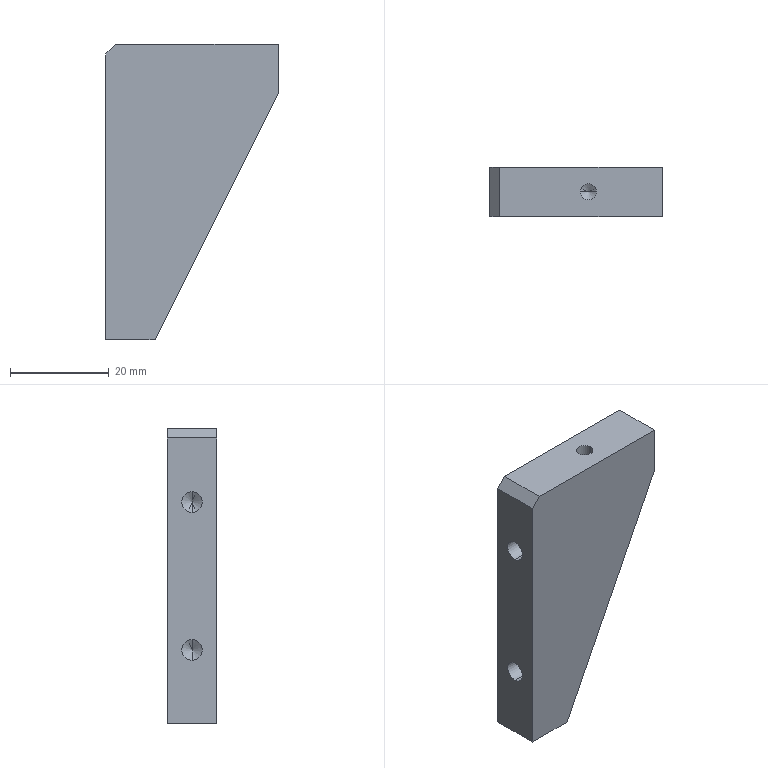Part | STEP file | PN_0051 | 1 solid | 20 faces | box 35 x 10 x 60 mm | volume 14229 mm3 | plane 8 | cylinder 6 | cone 6 | commonest cylinder face diameters 4.2 x4 3.3 x2
STEP:
#1=CARTESIAN_POINT('',(0.,0.,0.));
#2=DIRECTION('',(0.,0.,1.));
#3=DIRECTION('',(1.,0.,0.));
#4=AXIS2_PLACEMENT_3D('',#1,#2,#3);
#5=CARTESIAN_POINT('',(21.65,5.,-11.5));
#6=VERTEX_POINT('',#5);
#7=CARTESIAN_POINT('',(21.65,5.,0.));
#8=VERTEX_POINT('',#7);
#9=CARTESIAN_POINT('',(21.65,5.,0.));
#10=DIRECTION('',(0.,0.,1.));
#11=VECTOR('',#10,1.);
#12=LINE('',#9,#11);
#13=CARTESIAN_POINT('',(20.,5.,0.));
#14=DIRECTION('',(0.,0.,1.));
#15=DIRECTION('',(1.,0.,0.));
#16=AXIS2_PLACEMENT_3D('',#13,#14,#15);
#17=CYLINDRICAL_SURFACE('',#16,1.65);
#18=CARTESIAN_POINT('',(6.283,0.));
#19=DIRECTION('',(0.,1.));
#20=VECTOR('',#19,1.);
#21=LINE('',#18,#20);
#22=(GEOMETRIC_REPRESENTATION_CONTEXT(2)PARAMETRIC_REPRESENTATION_CONTEXT()REPRESENTATION_CONTEXT('',''));
#23=DEFINITIONAL_REPRESENTATION('',(#21),#22);
#24=PCURVE('',#17,#23);
#25=CARTESIAN_POINT('',(20.,5.,0.));
#26=DIRECTION('',(0.,0.,1.));
#27=DIRECTION('',(1.,0.,0.));
#28=AXIS2_PLACEMENT_3D('',#25,#26,#27);
#29=CYLINDRICAL_SURFACE('',#28,1.65);
#30=CARTESIAN_POINT('',(0.,0.));
#31=DIRECTION('',(0.,1.));
#32=VECTOR('',#31,1.);
#33=LINE('',#30,#32);
#34=(GEOMETRIC_REPRESENTATION_CONTEXT(2)PARAMETRIC_REPRESENTATION_CONTEXT()REPRESENTATION_CONTEXT('',''));
#35=DEFINITIONAL_REPRESENTATION('',(#33),#34);
#36=PCURVE('',#29,#35);
#37=SURFACE_CURVE('',#12,(#24,#36),.PCURVE_S1.);
#38=EDGE_CURVE('',#6,#8,#37,.T.);
#39=ORIENTED_EDGE('',*,*,#38,.T.);
#40=CARTESIAN_POINT('',(18.35,5.,0.));
#41=VERTEX_POINT('',#40);
#42=CARTESIAN_POINT('',(20.,5.,0.));
#43=DIRECTION('',(0.,0.,1.));
#44=DIRECTION('',(1.,0.,0.));
#45=AXIS2_PLACEMENT_3D('',#42,#43,#44);
#46=CIRCLE('',#45,1.65);
#47=CARTESIAN_POINT('',(0.,0.));
#48=DIRECTION('',(1.,0.));
#49=VECTOR('',#48,1.);
#50=LINE('',#47,#49);
#51=(GEOMETRIC_REPRESENTATION_CONTEXT(2)PARAMETRIC_REPRESENTATION_CONTEXT()REPRESENTATION_CONTEXT('',''));
#52=DEFINITIONAL_REPRESENTATION('',(#50),#51);
#53=PCURVE('',#17,#52);
#54=CARTESIAN_POINT('',(0.,10.,0.));
#55=DIRECTION('',(0.,0.,-1.));
#56=DIRECTION('',(-1.,0.,0.));
#57=AXIS2_PLACEMENT_3D('',#54,#55,#56);
#58=PLANE('',#57);
#59=CARTESIAN_POINT('',(-21.65,-5.));
#60=CARTESIAN_POINT('',(-21.65,-2.142));
#61=CARTESIAN_POINT('',(-19.175,-3.571));
#62=CARTESIAN_POINT('',(-16.7,-5.));
#63=CARTESIAN_POINT('',(-19.175,-6.429));
#64=CARTESIAN_POINT('',(-21.65,-7.858));
#65=CARTESIAN_POINT('',(-21.65,-5.));
#66=(BOUNDED_CURVE()B_SPLINE_CURVE(2,(#59,#60,#61,#62,#63,#64,#65),.UNSPECIFIED.,.T.,.F.)B_SPLINE_CURVE_WITH_KNOTS((1,2,2,2,2,1),(-2.094,0.,2.094,4.189,6.283,8.378),.UNSPECIFIED.)CURVE()GEOMETRIC_REPRESENTATION_ITEM()RATIONAL_B_SPLINE_CURVE((1.,0.5,1.,0.5,1.,0.5,1.))REPRESENTATION_ITEM(''));
#67=(GEOMETRIC_REPRESENTATION_CONTEXT(2)PARAMETRIC_REPRESENTATION_CONTEXT()REPRESENTATION_CONTEXT('',''));
#68=DEFINITIONAL_REPRESENTATION('',(#66),#67);
#69=PCURVE('',#58,#68);
#70=SURFACE_CURVE('',#46,(#53,#69),.PCURVE_S1.);
#71=EDGE_CURVE('',#41,#8,#70,.T.);
#72=ORIENTED_EDGE('',*,*,#71,.F.);
#73=CARTESIAN_POINT('',(18.35,5.,-11.5));
#74=VERTEX_POINT('',#73);
#75=CARTESIAN_POINT('',(18.35,5.,0.));
#76=DIRECTION('',(0.,0.,1.));
#77=VECTOR('',#76,1.);
#78=LINE('',#75,#77);
#79=CARTESIAN_POINT('',(3.142,0.));
#80=DIRECTION('',(0.,1.));
#81=VECTOR('',#80,1.);
#82=LINE('',#79,#81);
#83=(GEOMETRIC_REPRESENTATION_CONTEXT(2)PARAMETRIC_REPRESENTATION_CONTEXT()REPRESENTATION_CONTEXT('',''));
#84=DEFINITIONAL_REPRESENTATION('',(#82),#83);
#85=PCURVE('',#17,#84);
#86=CARTESIAN_POINT('',(3.142,0.));
#87=DIRECTION('',(0.,1.));
#88=VECTOR('',#87,1.);
#89=LINE('',#86,#88);
#90=(GEOMETRIC_REPRESENTATION_CONTEXT(2)PARAMETRIC_REPRESENTATION_CONTEXT()REPRESENTATION_CONTEXT('',''));
#91=DEFINITIONAL_REPRESENTATION('',(#89),#90);
#92=PCURVE('',#29,#91);
#93=SURFACE_CURVE('',#78,(#85,#92),.PCURVE_S1.);
#94=EDGE_CURVE('',#74,#41,#93,.T.);
#95=ORIENTED_EDGE('',*,*,#94,.F.);
#96=CARTESIAN_POINT('',(20.,5.,-11.5));
#97=DIRECTION('',(0.,0.,1.));
#98=DIRECTION('',(1.,0.,0.));
#99=AXIS2_PLACEMENT_3D('',#96,#97,#98);
#100=CIRCLE('',#99,1.65);
#101=CARTESIAN_POINT('',(0.,-11.5));
#102=DIRECTION('',(1.,0.));
#103=VECTOR('',#102,1.);
#104=LINE('',#101,#103);
#105=(GEOMETRIC_REPRESENTATION_CONTEXT(2)PARAMETRIC_REPRESENTATION_CONTEXT()REPRESENTATION_CONTEXT('',''));
#106=DEFINITIONAL_REPRESENTATION('',(#104),#105);
#107=PCURVE('',#17,#106);
#108=CARTESIAN_POINT('',(20.,5.,-11.5));
#109=DIRECTION('',(0.,0.,1.));
#110=DIRECTION('',(1.,0.,0.));
#111=AXIS2_PLACEMENT_3D('',#108,#109,#110);
#112=CONICAL_SURFACE('',#111,1.65,1.03);
#113=CARTESIAN_POINT('',(0.,0.));
#114=DIRECTION('',(1.,0.));
#115=VECTOR('',#114,1.);
#116=LINE('',#113,#115);
#117=(GEOMETRIC_REPRESENTATION_CONTEXT(2)PARAMETRIC_REPRESENTATION_CONTEXT()REPRESENTATION_CONTEXT('',''));
#118=DEFINITIONAL_REPRESENTATION('',(#116),#117);
#119=PCURVE('',#112,#118);
#120=SURFACE_CURVE('',#100,(#107,#119),.PCURVE_S1.);
#121=EDGE_CURVE('',#74,#6,#120,.T.);
#122=ORIENTED_EDGE('',*,*,#121,.T.);
#123=EDGE_LOOP('',(#39,#72,#95,#122));
#124=FACE_BOUND('',#123,.F.);
#125=ADVANCED_FACE('',(#124),#17,.F.);
#126=ORIENTED_EDGE('',*,*,#121,.F.);
#127=CARTESIAN_POINT('',(20.,5.,-12.491));
#128=VERTEX_POINT('',#127);
#129=CARTESIAN_POINT('',(18.35,5.,-11.5));
#130=DIRECTION('',(-0.8572,0.,0.515));
#131=VECTOR('',#130,1.);
#132=LINE('',#129,#131);
#133=CARTESIAN_POINT('',(3.142,0.));
#134=DIRECTION('',(0.,1.));
#135=VECTOR('',#134,1.);
#136=LINE('',#133,#135);
#137=(GEOMETRIC_REPRESENTATION_CONTEXT(2)PARAMETRIC_REPRESENTATION_CONTEXT()REPRESENTATION_CONTEXT('',''));
#138=DEFINITIONAL_REPRESENTATION('',(#136),#137);
#139=PCURVE('',#112,#138);
#140=CARTESIAN_POINT('',(20.,5.,-11.5));
#141=DIRECTION('',(0.,0.,1.));
#142=DIRECTION('',(1.,0.,0.));
#143=AXIS2_PLACEMENT_3D('',#140,#141,#142);
#144=CONICAL_SURFACE('',#143,1.65,1.03);
#145=CARTESIAN_POINT('',(3.142,0.));
#146=DIRECTION('',(0.,1.));
#147=VECTOR('',#146,1.);
#148=LINE('',#145,#147);
#149=(GEOMETRIC_REPRESENTATION_CONTEXT(2)PARAMETRIC_REPRESENTATION_CONTEXT()REPRESENTATION_CONTEXT('',''));
#150=DEFINITIONAL_REPRESENTATION('',(#148),#149);
#151=PCURVE('',#144,#150);
#152=SURFACE_CURVE('',#132,(#139,#151),.PCURVE_S1.);
#153=EDGE_CURVE('',#128,#74,#152,.T.);
#154=ORIENTED_EDGE('',*,*,#153,.F.);
#155=CARTESIAN_POINT('',(21.65,5.,-11.5));
#156=DIRECTION('',(0.8572,0.,0.515));
#157=VECTOR('',#156,1.);
#158=LINE('',#155,#157);
#159=CARTESIAN_POINT('',(6.283,0.));
#160=DIRECTION('',(0.,1.));
#161=VECTOR('',#160,1.);
#162=LINE('',#159,#161);
#163=(GEOMETRIC_REPRESENTATION_CONTEXT(2)PARAMETRIC_REPRESENTATION_CONTEXT()REPRESENTATION_CONTEXT('',''));
#164=DEFINITIONAL_REPRESENTATION('',(#162),#163);
#165=PCURVE('',#112,#164);
#166=CARTESIAN_POINT('',(0.,0.));
#167=DIRECTION('',(0.,1.));
#168=VECTOR('',#167,1.);
#169=LINE('',#166,#168);
#170=(GEOMETRIC_REPRESENTATION_CONTEXT(2)PARAMETRIC_REPRESENTATION_CONTEXT()REPRESENTATION_CONTEXT('',''));
#171=DEFINITIONAL_REPRESENTATION('',(#169),#170);
#172=PCURVE('',#144,#171);
#173=SURFACE_CURVE('',#158,(#165,#172),.PCURVE_S1.);
#174=EDGE_CURVE('',#128,#6,#173,.T.);
#175=ORIENTED_EDGE('',*,*,#174,.T.);
#176=EDGE_LOOP('',(#126,#154,#175));
#177=FACE_BOUND('',#176,.F.);
#178=ADVANCED_FACE('',(#177),#112,.F.);
#179=CARTESIAN_POINT('',(14.,5.,-42.9));
#180=VERTEX_POINT('',#179);
#181=CARTESIAN_POINT('',(0.,5.,-42.9));
#182=VERTEX_POINT('',#181);
#183=CARTESIAN_POINT('',(0.,5.,-42.9));
#184=DIRECTION('',(-1.,0.,0.));
#185=VECTOR('',#184,1.);
#186=LINE('',#183,#185);
#187=CARTESIAN_POINT('',(0.,5.,-45.));
#188=DIRECTION('',(-1.,0.,0.));
#189=DIRECTION('',(0.,0.,1.));
#190=AXIS2_PLACEMENT_3D('',#187,#188,#189);
#191=CYLINDRICAL_SURFACE('',#190,2.1);
#192=CARTESIAN_POINT('',(6.283,0.));
#193=DIRECTION('',(0.,1.));
#194=VECTOR('',#193,1.);
#195=LINE('',#192,#194);
#196=(GEOMETRIC_REPRESENTATION_CONTEXT(2)PARAMETRIC_REPRESENTATION_CONTEXT()REPRESENTATION_CONTEXT('',''));
#197=DEFINITIONAL_REPRESENTATION('',(#195),#196);
#198=PCURVE('',#191,#197);
#199=CARTESIAN_POINT('',(0.,5.,-45.));
#200=DIRECTION('',(-1.,0.,0.));
#201=DIRECTION('',(0.,0.,1.));
#202=AXIS2_PLACEMENT_3D('',#199,#200,#201);
#203=CYLINDRICAL_SURFACE('',#202,2.1);
#204=CARTESIAN_POINT('',(0.,0.));
#205=DIRECTION('',(0.,1.));
#206=VECTOR('',#205,1.);
#207=LINE('',#204,#206);
#208=(GEOMETRIC_REPRESENTATION_CONTEXT(2)PARAMETRIC_REPRESENTATION_CONTEXT()REPRESENTATION_CONTEXT('',''));
#209=DEFINITIONAL_REPRESENTATION('',(#207),#208);
#210=PCURVE('',#203,#209);
#211=SURFACE_CURVE('',#186,(#198,#210),.PCURVE_S1.);
#212=EDGE_CURVE('',#180,#182,#211,.T.);
#213=ORIENTED_EDGE('',*,*,#212,.T.);
#214=CARTESIAN_POINT('',(0.,5.,-47.1));
#215=VERTEX_POINT('',#214);
#216=CARTESIAN_POINT('',(0.,5.,-45.));
#217=DIRECTION('',(-1.,0.,0.));
#218=DIRECTION('',(0.,0.,1.));
#219=AXIS2_PLACEMENT_3D('',#216,#217,#218);
#220=CIRCLE('',#219,2.1);
#221=CARTESIAN_POINT('',(0.,0.));
#222=DIRECTION('',(1.,0.));
#223=VECTOR('',#222,1.);
#224=LINE('',#221,#223);
#225=(GEOMETRIC_REPRESENTATION_CONTEXT(2)PARAMETRIC_REPRESENTATION_CONTEXT()REPRESENTATION_CONTEXT('',''));
#226=DEFINITIONAL_REPRESENTATION('',(#224),#225);
#227=PCURVE('',#191,#226);
#228=CARTESIAN_POINT('',(0.,10.,-60.));
#229=DIRECTION('',(1.,0.,0.));
#230=DIRECTION('',(0.,0.,-1.));
#231=AXIS2_PLACEMENT_3D('',#228,#229,#230);
#232=PLANE('',#231);
#233=CARTESIAN_POINT('',(-17.1,-5.));
#234=CARTESIAN_POINT('',(-17.1,-1.363));
#235=CARTESIAN_POINT('',(-13.95,-3.181));
#236=CARTESIAN_POINT('',(-10.8,-5.));
#237=CARTESIAN_POINT('',(-13.95,-6.819));
#238=CARTESIAN_POINT('',(-17.1,-8.637));
#239=CARTESIAN_POINT('',(-17.1,-5.));
#240=(BOUNDED_CURVE()B_SPLINE_CURVE(2,(#233,#234,#235,#236,#237,#238,#239),.UNSPECIFIED.,.T.,.F.)B_SPLINE_CURVE_WITH_KNOTS((1,2,2,2,2,1),(-2.094,0.,2.094,4.189,6.283,8.378),.UNSPECIFIED.)CURVE()GEOMETRIC_REPRESENTATION_ITEM()RATIONAL_B_SPLINE_CURVE((1.,0.5,1.,0.5,1.,0.5,1.))REPRESENTATION_ITEM(''));
#241=(GEOMETRIC_REPRESENTATION_CONTEXT(2)PARAMETRIC_REPRESENTATION_CONTEXT()REPRESENTATION_CONTEXT('',''));
#242=DEFINITIONAL_REPRESENTATION('',(#240),#241);
#243=PCURVE('',#232,#242);
#244=SURFACE_CURVE('',#220,(#227,#243),.PCURVE_S1.);
#245=EDGE_CURVE('',#215,#182,#244,.T.);
#246=ORIENTED_EDGE('',*,*,#245,.F.);
#247=CARTESIAN_POINT('',(14.,5.,-47.1));
#248=VERTEX_POINT('',#247);
#249=CARTESIAN_POINT('',(0.,5.,-47.1));
#250=DIRECTION('',(-1.,0.,0.));
#251=VECTOR('',#250,1.);
#252=LINE('',#249,#251);
#253=CARTESIAN_POINT('',(3.142,0.));
#254=DIRECTION('',(0.,1.));
#255=VECTOR('',#254,1.);
#256=LINE('',#253,#255);
#257=(GEOMETRIC_REPRESENTATION_CONTEXT(2)PARAMETRIC_REPRESENTATION_CONTEXT()REPRESENTATION_CONTEXT('',''));
#258=DEFINITIONAL_REPRESENTATION('',(#256),#257);
#259=PCURVE('',#191,#258);
#260=CARTESIAN_POINT('',(3.142,0.));
#261=DIRECTION('',(0.,1.));
#262=VECTOR('',#261,1.);
#263=LINE('',#260,#262);
#264=(GEOMETRIC_REPRESENTATION_CONTEXT(2)PARAMETRIC_REPRESENTATION_CONTEXT()REPRESENTATION_CONTEXT('',''));
#265=DEFINITIONAL_REPRESENTATION('',(#263),#264);
#266=PCURVE('',#203,#265);
#267=SURFACE_CURVE('',#252,(#259,#266),.PCURVE_S1.);
#268=EDGE_CURVE('',#248,#215,#267,.T.);
#269=ORIENTED_EDGE('',*,*,#268,.F.);
#270=CARTESIAN_POINT('',(14.,5.,-45.));
#271=DIRECTION('',(-1.,0.,0.));
#272=DIRECTION('',(0.,0.,1.));
#273=AXIS2_PLACEMENT_3D('',#270,#271,#272);
#274=CIRCLE('',#273,2.1);
#275=CARTESIAN_POINT('',(0.,-14.));
#276=DIRECTION('',(1.,0.));
#277=VECTOR('',#276,1.);
#278=LINE('',#275,#277);
#279=(GEOMETRIC_REPRESENTATION_CONTEXT(2)PARAMETRIC_REPRESENTATION_CONTEXT()REPRESENTATION_CONTEXT('',''));
#280=DEFINITIONAL_REPRESENTATION('',(#278),#279);
#281=PCURVE('',#191,#280);
#282=CARTESIAN_POINT('',(14.,5.,-45.));
#283=DIRECTION('',(-1.,0.,0.));
#284=DIRECTION('',(0.,0.,1.));
#285=AXIS2_PLACEMENT_3D('',#282,#283,#284);
#286=CONICAL_SURFACE('',#285,2.1,1.03);
#287=CARTESIAN_POINT('',(0.,0.));
#288=DIRECTION('',(1.,0.));
#289=VECTOR('',#288,1.);
#290=LINE('',#287,#289);
#291=(GEOMETRIC_REPRESENTATION_CONTEXT(2)PARAMETRIC_REPRESENTATION_CONTEXT()REPRESENTATION_CONTEXT('',''));
#292=DEFINITIONAL_REPRESENTATION('',(#290),#291);
#293=PCURVE('',#286,#292);
#294=SURFACE_CURVE('',#274,(#281,#293),.PCURVE_S1.);
#295=EDGE_CURVE('',#248,#180,#294,.T.);
#296=ORIENTED_EDGE('',*,*,#295,.T.);
#297=EDGE_LOOP('',(#213,#246,#269,#296));
#298=FACE_BOUND('',#297,.F.);
#299=ADVANCED_FACE('',(#298),#191,.F.);
#300=ORIENTED_EDGE('',*,*,#295,.F.);
#301=CARTESIAN_POINT('',(15.262,5.,-45.));
#302=VERTEX_POINT('',#301);
#303=CARTESIAN_POINT('',(14.,5.,-47.1));
#304=DIRECTION('',(-0.515,0.,-0.8572));
#305=VECTOR('',#304,1.);
#306=LINE('',#303,#305);
#307=CARTESIAN_POINT('',(3.142,-1.262));
#308=CARTESIAN_POINT('',(3.142,-1.243));
#309=CARTESIAN_POINT('',(3.142,-1.204));
#310=CARTESIAN_POINT('',(3.142,-1.147));
#311=CARTESIAN_POINT('',(3.142,-1.09));
#312=CARTESIAN_POINT('',(3.142,-1.032));
#313=CARTESIAN_POINT('',(3.142,-0.975));
#314=CARTESIAN_POINT('',(3.142,-0.9177));
#315=CARTESIAN_POINT('',(3.142,-0.8603));
#316=CARTESIAN_POINT('',(3.142,-0.803));
#317=CARTESIAN_POINT('',(3.142,-0.7456));
#318=CARTESIAN_POINT('',(3.142,-0.6883));
#319=CARTESIAN_POINT('',(3.142,-0.6309));
#320=CARTESIAN_POINT('',(3.142,-0.5735));
#321=CARTESIAN_POINT('',(3.142,-0.5162));
#322=CARTESIAN_POINT('',(3.142,-0.4588));
#323=CARTESIAN_POINT('',(3.142,-0.4015));
#324=CARTESIAN_POINT('',(3.142,-0.3441));
#325=CARTESIAN_POINT('',(3.142,-0.2868));
#326=CARTESIAN_POINT('',(3.142,-0.2294));
#327=CARTESIAN_POINT('',(3.142,-0.1721));
#328=CARTESIAN_POINT('',(3.142,-0.1147));
#329=CARTESIAN_POINT('',(3.142,-0.05735));
#330=CARTESIAN_POINT('',(3.142,-0.01912));
#331=CARTESIAN_POINT('',(3.142,0.));
#332=B_SPLINE_CURVE_WITH_KNOTS('',3,(#307,#308,#309,#310,#311,#312,#313,#314,#315,#316,#317,#318,#319,#320,#321,#322,#323,#324,#325,#326,#327,#328,#329,#330,#331),.UNSPECIFIED.,.F.,.F.,(4,1,1,1,1,1,1,1,1,1,1,1,1,1,1,1,1,1,1,1,1,1,4),(-2.45,-2.339,-2.227,-2.116,-2.004,-1.893,-1.782,-1.67,-1.559,-1.448,-1.336,-1.225,-1.114,-1.002,-0.8909,-0.7795,-0.6682,-0.5568,-0.4454,-0.3341,-0.2227,-0.1114,0.),.UNSPECIFIED.);
#333=(GEOMETRIC_REPRESENTATION_CONTEXT(2)PARAMETRIC_REPRESENTATION_CONTEXT()REPRESENTATION_CONTEXT('',''));
#334=DEFINITIONAL_REPRESENTATION('',(#332),#333);
#335=PCURVE('',#286,#334);
#336=CARTESIAN_POINT('',(14.,5.,-45.));
#337=DIRECTION('',(-1.,0.,0.));
#338=DIRECTION('',(0.,0.,1.));
#339=AXIS2_PLACEMENT_3D('',#336,#337,#338);
#340=CONICAL_SURFACE('',#339,2.1,1.03);
#341=CARTESIAN_POINT('',(3.142,-1.262));
#342=CARTESIAN_POINT('',(3.142,-1.243));
#343=CARTESIAN_POINT('',(3.142,-1.204));
#344=CARTESIAN_POINT('',(3.142,-1.147));
#345=CARTESIAN_POINT('',(3.142,-1.09));
#346=CARTESIAN_POINT('',(3.142,-1.032));
#347=CARTESIAN_POINT('',(3.142,-0.975));
#348=CARTESIAN_POINT('',(3.142,-0.9177));
#349=CARTESIAN_POINT('',(3.142,-0.8603));
#350=CARTESIAN_POINT('',(3.142,-0.803));
#351=CARTESIAN_POINT('',(3.142,-0.7456));
#352=CARTESIAN_POINT('',(3.142,-0.6883));
#353=CARTESIAN_POINT('',(3.142,-0.6309));
#354=CARTESIAN_POINT('',(3.142,-0.5735));
#355=CARTESIAN_POINT('',(3.142,-0.5162));
#356=CARTESIAN_POINT('',(3.142,-0.4588));
#357=CARTESIAN_POINT('',(3.142,-0.4015));
#358=CARTESIAN_POINT('',(3.142,-0.3441));
#359=CARTESIAN_POINT('',(3.142,-0.2868));
#360=CARTESIAN_POINT('',(3.142,-0.2294));
#361=CARTESIAN_POINT('',(3.142,-0.1721));
#362=CARTESIAN_POINT('',(3.142,-0.1147));
#363=CARTESIAN_POINT('',(3.142,-0.05735));
#364=CARTESIAN_POINT('',(3.142,-0.01912));
#365=CARTESIAN_POINT('',(3.142,0.));
#366=B_SPLINE_CURVE_WITH_KNOTS('',3,(#341,#342,#343,#344,#345,#346,#347,#348,#349,#350,#351,#352,#353,#354,#355,#356,#357,#358,#359,#360,#361,#362,#363,#364,#365),.UNSPECIFIED.,.F.,.F.,(4,1,1,1,1,1,1,1,1,1,1,1,1,1,1,1,1,1,1,1,1,1,4),(-2.45,-2.339,-2.227,-2.116,-2.004,-1.893,-1.782,-1.67,-1.559,-1.448,-1.336,-1.225,-1.114,-1.002,-0.8909,-0.7795,-0.6682,-0.5568,-0.4454,-0.3341,-0.2227,-0.1114,0.),.UNSPECIFIED.);
#367=(GEOMETRIC_REPRESENTATION_CONTEXT(2)PARAMETRIC_REPRESENTATION_CONTEXT()REPRESENTATION_CONTEXT('',''));
#368=DEFINITIONAL_REPRESENTATION('',(#366),#367);
#369=PCURVE('',#340,#368);
#370=SURFACE_CURVE('',#306,(#335,#369),.PCURVE_S1.);
#371=EDGE_CURVE('',#302,#248,#370,.T.);
#372=ORIENTED_EDGE('',*,*,#371,.F.);
#373=CARTESIAN_POINT('',(14.,5.,-42.9));
#374=DIRECTION('',(-0.515,0.,0.8572));
#375=VECTOR('',#374,1.);
#376=LINE('',#373,#375);
#377=CARTESIAN_POINT('',(6.283,0.));
#378=DIRECTION('',(0.,1.));
#379=VECTOR('',#378,1.);
#380=LINE('',#377,#379);
#381=(GEOMETRIC_REPRESENTATION_CONTEXT(2)PARAMETRIC_REPRESENTATION_CONTEXT()REPRESENTATION_CONTEXT('',''));
#382=DEFINITIONAL_REPRESENTATION('',(#380),#381);
#383=PCURVE('',#286,#382);
#384=CARTESIAN_POINT('',(0.,0.));
#385=DIRECTION('',(0.,1.));
#386=VECTOR('',#385,1.);
#387=LINE('',#384,#386);
#388=(GEOMETRIC_REPRESENTATION_CONTEXT(2)PARAMETRIC_REPRESENTATION_CONTEXT()REPRESENTATION_CONTEXT('',''));
#389=DEFINITIONAL_REPRESENTATION('',(#387),#388);
#390=PCURVE('',#340,#389);
#391=SURFACE_CURVE('',#376,(#383,#390),.PCURVE_S1.);
#392=EDGE_CURVE('',#302,#180,#391,.T.);
#393=ORIENTED_EDGE('',*,*,#392,.T.);
#394=EDGE_LOOP('',(#300,#372,#393));
#395=FACE_BOUND('',#394,.F.);
#396=ADVANCED_FACE('',(#395),#286,.F.);
#397=CARTESIAN_POINT('',(14.,5.,-12.9));
#398=VERTEX_POINT('',#397);
#399=CARTESIAN_POINT('',(0.,5.,-12.9));
#400=VERTEX_POINT('',#399);
#401=CARTESIAN_POINT('',(0.,5.,-12.9));
#402=DIRECTION('',(-1.,0.,0.));
#403=VECTOR('',#402,1.);
#404=LINE('',#401,#403);
#405=CARTESIAN_POINT('',(0.,5.,-15.));
#406=DIRECTION('',(-1.,0.,0.));
#407=DIRECTION('',(0.,0.,1.));
#408=AXIS2_PLACEMENT_3D('',#405,#406,#407);
#409=CYLINDRICAL_SURFACE('',#408,2.1);
#410=CARTESIAN_POINT('',(6.283,0.));
#411=DIRECTION('',(0.,1.));
#412=VECTOR('',#411,1.);
#413=LINE('',#410,#412);
#414=(GEOMETRIC_REPRESENTATION_CONTEXT(2)PARAMETRIC_REPRESENTATION_CONTEXT()REPRESENTATION_CONTEXT('',''));
#415=DEFINITIONAL_REPRESENTATION('',(#413),#414);
#416=PCURVE('',#409,#415);
#417=CARTESIAN_POINT('',(0.,5.,-15.));
#418=DIRECTION('',(-1.,0.,0.));
#419=DIRECTION('',(0.,0.,1.));
#420=AXIS2_PLACEMENT_3D('',#417,#418,#419);
#421=CYLINDRICAL_SURFACE('',#420,2.1);
#422=CARTESIAN_POINT('',(0.,0.));
#423=DIRECTION('',(0.,1.));
#424=VECTOR('',#423,1.);
#425=LINE('',#422,#424);
#426=(GEOMETRIC_REPRESENTATION_CONTEXT(2)PARAMETRIC_REPRESENTATION_CONTEXT()REPRESENTATION_CONTEXT('',''));
#427=DEFINITIONAL_REPRESENTATION('',(#425),#426);
#428=PCURVE('',#421,#427);
#429=SURFACE_CURVE('',#404,(#416,#428),.PCURVE_S1.);
#430=EDGE_CURVE('',#398,#400,#429,.T.);
#431=ORIENTED_EDGE('',*,*,#430,.T.);
#432=CARTESIAN_POINT('',(0.,5.,-17.1));
#433=VERTEX_POINT('',#432);
#434=CARTESIAN_POINT('',(0.,5.,-15.));
#435=DIRECTION('',(-1.,0.,0.));
#436=DIRECTION('',(0.,0.,1.));
#437=AXIS2_PLACEMENT_3D('',#434,#435,#436);
#438=CIRCLE('',#437,2.1);
#439=CARTESIAN_POINT('',(0.,0.));
#440=DIRECTION('',(1.,0.));
#441=VECTOR('',#440,1.);
#442=LINE('',#439,#441);
#443=(GEOMETRIC_REPRESENTATION_CONTEXT(2)PARAMETRIC_REPRESENTATION_CONTEXT()REPRESENTATION_CONTEXT('',''));
#444=DEFINITIONAL_REPRESENTATION('',(#442),#443);
#445=PCURVE('',#409,#444);
#446=CARTESIAN_POINT('',(-47.1,-5.));
#447=CARTESIAN_POINT('',(-47.1,-1.363));
#448=CARTESIAN_POINT('',(-43.95,-3.181));
#449=CARTESIAN_POINT('',(-40.8,-5.));
#450=CARTESIAN_POINT('',(-43.95,-6.819));
#451=CARTESIAN_POINT('',(-47.1,-8.637));
#452=CARTESIAN_POINT('',(-47.1,-5.));
#453=(BOUNDED_CURVE()B_SPLINE_CURVE(2,(#446,#447,#448,#449,#450,#451,#452),.UNSPECIFIED.,.T.,.F.)B_SPLINE_CURVE_WITH_KNOTS((1,2,2,2,2,1),(-2.094,0.,2.094,4.189,6.283,8.378),.UNSPECIFIED.)CURVE()GEOMETRIC_REPRESENTATION_ITEM()RATIONAL_B_SPLINE_CURVE((1.,0.5,1.,0.5,1.,0.5,1.))REPRESENTATION_ITEM(''));
#454=(GEOMETRIC_REPRESENTATION_CONTEXT(2)PARAMETRIC_REPRESENTATION_CONTEXT()REPRESENTATION_CONTEXT('',''));
#455=DEFINITIONAL_REPRESENTATION('',(#453),#454);
#456=PCURVE('',#232,#455);
#457=SURFACE_CURVE('',#438,(#445,#456),.PCURVE_S1.);
#458=EDGE_CURVE('',#433,#400,#457,.T.);
#459=ORIENTED_EDGE('',*,*,#458,.F.);
#460=CARTESIAN_POINT('',(14.,5.,-17.1));
#461=VERTEX_POINT('',#460);
#462=CARTESIAN_POINT('',(0.,5.,-17.1));
#463=DIRECTION('',(-1.,0.,0.));
#464=VECTOR('',#463,1.);
#465=LINE('',#462,#464);
#466=CARTESIAN_POINT('',(3.142,0.));
#467=DIRECTION('',(0.,1.));
#468=VECTOR('',#467,1.);
#469=LINE('',#466,#468);
#470=(GEOMETRIC_REPRESENTATION_CONTEXT(2)PARAMETRIC_REPRESENTATION_CONTEXT()REPRESENTATION_CONTEXT('',''));
#471=DEFINITIONAL_REPRESENTATION('',(#469),#470);
#472=PCURVE('',#409,#471);
#473=CARTESIAN_POINT('',(3.142,0.));
#474=DIRECTION('',(0.,1.));
#475=VECTOR('',#474,1.);
#476=LINE('',#473,#475);
#477=(GEOMETRIC_REPRESENTATION_CONTEXT(2)PARAMETRIC_REPRESENTATION_CONTEXT()REPRESENTATION_CONTEXT('',''));
#478=DEFINITIONAL_REPRESENTATION('',(#476),#477);
#479=PCURVE('',#421,#478);
#480=SURFACE_CURVE('',#465,(#472,#479),.PCURVE_S1.);
#481=EDGE_CURVE('',#461,#433,#480,.T.);
#482=ORIENTED_EDGE('',*,*,#481,.F.);
#483=CARTESIAN_POINT('',(14.,5.,-15.));
#484=DIRECTION('',(-1.,0.,0.));
#485=DIRECTION('',(0.,0.,1.));
#486=AXIS2_PLACEMENT_3D('',#483,#484,#485);
#487=CIRCLE('',#486,2.1);
#488=CARTESIAN_POINT('',(0.,-14.));
#489=DIRECTION('',(1.,0.));
#490=VECTOR('',#489,1.);
#491=LINE('',#488,#490);
#492=(GEOMETRIC_REPRESENTATION_CONTEXT(2)PARAMETRIC_REPRESENTATION_CONTEXT()REPRESENTATION_CONTEXT('',''));
#493=DEFINITIONAL_REPRESENTATION('',(#491),#492);
#494=PCURVE('',#409,#493);
#495=CARTESIAN_POINT('',(14.,5.,-15.));
#496=DIRECTION('',(-1.,0.,0.));
#497=DIRECTION('',(0.,0.,1.));
#498=AXIS2_PLACEMENT_3D('',#495,#496,#497);
#499=CONICAL_SURFACE('',#498,2.1,1.03);
#500=CARTESIAN_POINT('',(0.,0.));
#501=DIRECTION('',(1.,0.));
#502=VECTOR('',#501,1.);
#503=LINE('',#500,#502);
#504=(GEOMETRIC_REPRESENTATION_CONTEXT(2)PARAMETRIC_REPRESENTATION_CONTEXT()REPRESENTATION_CONTEXT('',''));
#505=DEFINITIONAL_REPRESENTATION('',(#503),#504);
#506=PCURVE('',#499,#505);
#507=SURFACE_CURVE('',#487,(#494,#506),.PCURVE_S1.);
#508=EDGE_CURVE('',#461,#398,#507,.T.);
#509=ORIENTED_EDGE('',*,*,#508,.T.);
#510=EDGE_LOOP('',(#431,#459,#482,#509));
#511=FACE_BOUND('',#510,.F.);
#512=ADVANCED_FACE('',(#511),#409,.F.);
#513=ORIENTED_EDGE('',*,*,#508,.F.);
#514=CARTESIAN_POINT('',(15.262,5.,-15.));
#515=VERTEX_POINT('',#514);
#516=CARTESIAN_POINT('',(14.,5.,-17.1));
#517=DIRECTION('',(-0.515,0.,-0.8572));
#518=VECTOR('',#517,1.);
#519=LINE('',#516,#518);
#520=CARTESIAN_POINT('',(3.142,-1.262));
#521=CARTESIAN_POINT('',(3.142,-1.243));
#522=CARTESIAN_POINT('',(3.142,-1.204));
#523=CARTESIAN_POINT('',(3.142,-1.147));
#524=CARTESIAN_POINT('',(3.142,-1.09));
#525=CARTESIAN_POINT('',(3.142,-1.032));
#526=CARTESIAN_POINT('',(3.142,-0.975));
#527=CARTESIAN_POINT('',(3.142,-0.9177));
#528=CARTESIAN_POINT('',(3.142,-0.8603));
#529=CARTESIAN_POINT('',(3.142,-0.803));
#530=CARTESIAN_POINT('',(3.142,-0.7456));
#531=CARTESIAN_POINT('',(3.142,-0.6883));
#532=CARTESIAN_POINT('',(3.142,-0.6309));
#533=CARTESIAN_POINT('',(3.142,-0.5735));
#534=CARTESIAN_POINT('',(3.142,-0.5162));
#535=CARTESIAN_POINT('',(3.142,-0.4588));
#536=CARTESIAN_POINT('',(3.142,-0.4015));
#537=CARTESIAN_POINT('',(3.142,-0.3441));
#538=CARTESIAN_POINT('',(3.142,-0.2868));
#539=CARTESIAN_POINT('',(3.142,-0.2294));
#540=CARTESIAN_POINT('',(3.142,-0.1721));
#541=CARTESIAN_POINT('',(3.142,-0.1147));
#542=CARTESIAN_POINT('',(3.142,-0.05735));
#543=CARTESIAN_POINT('',(3.142,-0.01912));
#544=CARTESIAN_POINT('',(3.142,0.));
#545=B_SPLINE_CURVE_WITH_KNOTS('',3,(#520,#521,#522,#523,#524,#525,#526,#527,#528,#529,#530,#531,#532,#533,#534,#535,#536,#537,#538,#539,#540,#541,#542,#543,#544),.UNSPECIFIED.,.F.,.F.,(4,1,1,1,1,1,1,1,1,1,1,1,1,1,1,1,1,1,1,1,1,1,4),(-2.45,-2.339,-2.227,-2.116,-2.004,-1.893,-1.782,-1.67,-1.559,-1.448,-1.336,-1.225,-1.114,-1.002,-0.8909,-0.7795,-0.6682,-0.5568,-0.4454,-0.3341,-0.2227,-0.1114,0.),.UNSPECIFIED.);
#546=(GEOMETRIC_REPRESENTATION_CONTEXT(2)PARAMETRIC_REPRESENTATION_CONTEXT()REPRESENTATION_CONTEXT('',''));
#547=DEFINITIONAL_REPRESENTATION('',(#545),#546);
#548=PCURVE('',#499,#547);
#549=CARTESIAN_POINT('',(14.,5.,-15.));
#550=DIRECTION('',(-1.,0.,0.));
#551=DIRECTION('',(0.,0.,1.));
#552=AXIS2_PLACEMENT_3D('',#549,#550,#551);
#553=CONICAL_SURFACE('',#552,2.1,1.03);
#554=CARTESIAN_POINT('',(3.142,-1.262));
#555=CARTESIAN_POINT('',(3.142,-1.243));
#556=CARTESIAN_POINT('',(3.142,-1.204));
#557=CARTESIAN_POINT('',(3.142,-1.147));
#558=CARTESIAN_POINT('',(3.142,-1.09));
#559=CARTESIAN_POINT('',(3.142,-1.032));
#560=CARTESIAN_POINT('',(3.142,-0.975));
#561=CARTESIAN_POINT('',(3.142,-0.9177));
#562=CARTESIAN_POINT('',(3.142,-0.8603));
#563=CARTESIAN_POINT('',(3.142,-0.803));
#564=CARTESIAN_POINT('',(3.142,-0.7456));
#565=CARTESIAN_POINT('',(3.142,-0.6883));
#566=CARTESIAN_POINT('',(3.142,-0.6309));
#567=CARTESIAN_POINT('',(3.142,-0.5735));
#568=CARTESIAN_POINT('',(3.142,-0.5162));
#569=CARTESIAN_POINT('',(3.142,-0.4588));
#570=CARTESIAN_POINT('',(3.142,-0.4015));
#571=CARTESIAN_POINT('',(3.142,-0.3441));
#572=CARTESIAN_POINT('',(3.142,-0.2868));
#573=CARTESIAN_POINT('',(3.142,-0.2294));
#574=CARTESIAN_POINT('',(3.142,-0.1721));
#575=CARTESIAN_POINT('',(3.142,-0.1147));
#576=CARTESIAN_POINT('',(3.142,-0.05735));
#577=CARTESIAN_POINT('',(3.142,-0.01912));
#578=CARTESIAN_POINT('',(3.142,0.));
#579=B_SPLINE_CURVE_WITH_KNOTS('',3,(#554,#555,#556,#557,#558,#559,#560,#561,#562,#563,#564,#565,#566,#567,#568,#569,#570,#571,#572,#573,#574,#575,#576,#577,#578),.UNSPECIFIED.,.F.,.F.,(4,1,1,1,1,1,1,1,1,1,1,1,1,1,1,1,1,1,1,1,1,1,4),(-2.45,-2.339,-2.227,-2.116,-2.004,-1.893,-1.782,-1.67,-1.559,-1.448,-1.336,-1.225,-1.114,-1.002,-0.8909,-0.7795,-0.6682,-0.5568,-0.4454,-0.3341,-0.2227,-0.1114,0.),.UNSPECIFIED.);
#580=(GEOMETRIC_REPRESENTATION_CONTEXT(2)PARAMETRIC_REPRESENTATION_CONTEXT()REPRESENTATION_CONTEXT('',''));
#581=DEFINITIONAL_REPRESENTATION('',(#579),#580);
#582=PCURVE('',#553,#581);
#583=SURFACE_CURVE('',#519,(#548,#582),.PCURVE_S1.);
#584=EDGE_CURVE('',#515,#461,#583,.T.);
#585=ORIENTED_EDGE('',*,*,#584,.F.);
#586=CARTESIAN_POINT('',(14.,5.,-12.9));
#587=DIRECTION('',(-0.515,0.,0.8572));
#588=VECTOR('',#587,1.);
#589=LINE('',#586,#588);
#590=CARTESIAN_POINT('',(6.283,0.));
#591=DIRECTION('',(0.,1.));
#592=VECTOR('',#591,1.);
#593=LINE('',#590,#592);
#594=(GEOMETRIC_REPRESENTATION_CONTEXT(2)PARAMETRIC_REPRESENTATION_CONTEXT()REPRESENTATION_CONTEXT('',''));
#595=DEFINITIONAL_REPRESENTATION('',(#593),#594);
#596=PCURVE('',#499,#595);
#597=CARTESIAN_POINT('',(0.,0.));
#598=DIRECTION('',(0.,1.));
#599=VECTOR('',#598,1.);
#600=LINE('',#597,#599);
#601=(GEOMETRIC_REPRESENTATION_CONTEXT(2)PARAMETRIC_REPRESENTATION_CONTEXT()REPRESENTATION_CONTEXT('',''));
#602=DEFINITIONAL_REPRESENTATION('',(#600),#601);
#603=PCURVE('',#553,#602);
#604=SURFACE_CURVE('',#589,(#596,#603),.PCURVE_S1.);
#605=EDGE_CURVE('',#515,#398,#604,.T.);
#606=ORIENTED_EDGE('',*,*,#605,.T.);
#607=EDGE_LOOP('',(#513,#585,#606));
#608=FACE_BOUND('',#607,.F.);
#609=ADVANCED_FACE('',(#608),#499,.F.);
#610=CARTESIAN_POINT('',(0.,5.,-45.));
#611=DIRECTION('',(-1.,0.,0.));
#612=DIRECTION('',(0.,0.,1.));
#613=AXIS2_PLACEMENT_3D('',#610,#611,#612);
#614=CIRCLE('',#613,2.1);
#615=CARTESIAN_POINT('',(-17.1,-5.));
#616=CARTESIAN_POINT('',(-17.1,-1.363));
#617=CARTESIAN_POINT('',(-13.95,-3.181));
#618=CARTESIAN_POINT('',(-10.8,-5.));
#619=CARTESIAN_POINT('',(-13.95,-6.819));
#620=CARTESIAN_POINT('',(-17.1,-8.637));
#621=CARTESIAN_POINT('',(-17.1,-5.));
#622=(BOUNDED_CURVE()B_SPLINE_CURVE(2,(#615,#616,#617,#618,#619,#620,#621),.UNSPECIFIED.,.T.,.F.)B_SPLINE_CURVE_WITH_KNOTS((1,2,2,2,2,1),(-2.094,0.,2.094,4.189,6.283,8.378),.UNSPECIFIED.)CURVE()GEOMETRIC_REPRESENTATION_ITEM()RATIONAL_B_SPLINE_CURVE((1.,0.5,1.,0.5,1.,0.5,1.))REPRESENTATION_ITEM(''));
#623=(GEOMETRIC_REPRESENTATION_CONTEXT(2)PARAMETRIC_REPRESENTATION_CONTEXT()REPRESENTATION_CONTEXT('',''));
#624=DEFINITIONAL_REPRESENTATION('',(#622),#623);
#625=PCURVE('',#232,#624);
#626=CARTESIAN_POINT('',(0.,0.));
#627=DIRECTION('',(1.,0.));
#628=VECTOR('',#627,1.);
#629=LINE('',#626,#628);
#630=(GEOMETRIC_REPRESENTATION_CONTEXT(2)PARAMETRIC_REPRESENTATION_CONTEXT()REPRESENTATION_CONTEXT('',''));
#631=DEFINITIONAL_REPRESENTATION('',(#629),#630);
#632=PCURVE('',#203,#631);
#633=SURFACE_CURVE('',#614,(#625,#632),.PCURVE_S1.);
#634=EDGE_CURVE('',#182,#215,#633,.T.);
#635=ORIENTED_EDGE('',*,*,#634,.F.);
#636=ORIENTED_EDGE('',*,*,#245,.F.);
#637=EDGE_LOOP('',(#635,#636));
#638=FACE_BOUND('',#637,.T.);
#639=CARTESIAN_POINT('',(0.,5.,-15.));
#640=DIRECTION('',(-1.,0.,0.));
#641=DIRECTION('',(0.,0.,1.));
#642=AXIS2_PLACEMENT_3D('',#639,#640,#641);
#643=CIRCLE('',#642,2.1);
#644=CARTESIAN_POINT('',(-47.1,-5.));
#645=CARTESIAN_POINT('',(-47.1,-1.363));
#646=CARTESIAN_POINT('',(-43.95,-3.181));
#647=CARTESIAN_POINT('',(-40.8,-5.));
#648=CARTESIAN_POINT('',(-43.95,-6.819));
#649=CARTESIAN_POINT('',(-47.1,-8.637));
#650=CARTESIAN_POINT('',(-47.1,-5.));
#651=(BOUNDED_CURVE()B_SPLINE_CURVE(2,(#644,#645,#646,#647,#648,#649,#650),.UNSPECIFIED.,.T.,.F.)B_SPLINE_CURVE_WITH_KNOTS((1,2,2,2,2,1),(-2.094,0.,2.094,4.189,6.283,8.378),.UNSPECIFIED.)CURVE()GEOMETRIC_REPRESENTATION_ITEM()RATIONAL_B_SPLINE_CURVE((1.,0.5,1.,0.5,1.,0.5,1.))REPRESENTATION_ITEM(''));
#652=(GEOMETRIC_REPRESENTATION_CONTEXT(2)PARAMETRIC_REPRESENTATION_CONTEXT()REPRESENTATION_CONTEXT('',''));
#653=DEFINITIONAL_REPRESENTATION('',(#651),#652);
#654=PCURVE('',#232,#653);
#655=CARTESIAN_POINT('',(0.,0.));
#656=DIRECTION('',(1.,0.));
#657=VECTOR('',#656,1.);
#658=LINE('',#655,#657);
#659=(GEOMETRIC_REPRESENTATION_CONTEXT(2)PARAMETRIC_REPRESENTATION_CONTEXT()REPRESENTATION_CONTEXT('',''));
#660=DEFINITIONAL_REPRESENTATION('',(#658),#659);
#661=PCURVE('',#421,#660);
#662=SURFACE_CURVE('',#643,(#654,#661),.PCURVE_S1.);
#663=EDGE_CURVE('',#400,#433,#662,.T.);
#664=ORIENTED_EDGE('',*,*,#663,.F.);
#665=ORIENTED_EDGE('',*,*,#458,.F.);
#666=EDGE_LOOP('',(#664,#665));
#667=FACE_BOUND('',#666,.T.);
#668=CARTESIAN_POINT('',(0.,0.,-60.));
#669=VERTEX_POINT('',#668);
#670=CARTESIAN_POINT('',(0.,0.,-2.));
#671=VERTEX_POINT('',#670);
#672=CARTESIAN_POINT('',(0.,0.,-60.));
#673=DIRECTION('',(0.,0.,1.));
#674=VECTOR('',#673,1.);
#675=LINE('',#672,#674);
#676=CARTESIAN_POINT('',(0.,-10.));
#677=DIRECTION('',(-1.,0.));
#678=VECTOR('',#677,1.);
#679=LINE('',#676,#678);
#680=(GEOMETRIC_REPRESENTATION_CONTEXT(2)PARAMETRIC_REPRESENTATION_CONTEXT()REPRESENTATION_CONTEXT('',''));
#681=DEFINITIONAL_REPRESENTATION('',(#679),#680);
#682=PCURVE('',#232,#681);
#683=CARTESIAN_POINT('',(0.,0.,0.));
#684=DIRECTION('',(0.,1.,0.));
#685=DIRECTION('',(0.,0.,1.));
#686=AXIS2_PLACEMENT_3D('',#683,#684,#685);
#687=PLANE('',#686);
#688=CARTESIAN_POINT('',(-60.,0.));
#689=DIRECTION('',(1.,0.));
#690=VECTOR('',#689,1.);
#691=LINE('',#688,#690);
#692=(GEOMETRIC_REPRESENTATION_CONTEXT(2)PARAMETRIC_REPRESENTATION_CONTEXT()REPRESENTATION_CONTEXT('',''));
#693=DEFINITIONAL_REPRESENTATION('',(#691),#692);
#694=PCURVE('',#687,#693);
#695=SURFACE_CURVE('',#675,(#682,#694),.PCURVE_S1.);
#696=EDGE_CURVE('',#669,#671,#695,.T.);
#697=ORIENTED_EDGE('',*,*,#696,.T.);
#698=CARTESIAN_POINT('',(0.,10.,-2.));
#699=VERTEX_POINT('',#698);
#700=CARTESIAN_POINT('',(0.,10.,-2.));
#701=DIRECTION('',(0.,1.,0.));
#702=VECTOR('',#701,1.);
#703=LINE('',#700,#702);
#704=CARTESIAN_POINT('',(-58.,0.));
#705=DIRECTION('',(0.,1.));
#706=VECTOR('',#705,1.);
#707=LINE('',#704,#706);
#708=(GEOMETRIC_REPRESENTATION_CONTEXT(2)PARAMETRIC_REPRESENTATION_CONTEXT()REPRESENTATION_CONTEXT('',''));
#709=DEFINITIONAL_REPRESENTATION('',(#707),#708);
#710=PCURVE('',#232,#709);
#711=CARTESIAN_POINT('',(2.,10.,0.));
#712=DIRECTION('',(0.7071,0.,-0.7071));
#713=DIRECTION('',(0.,-1.,0.));
#714=AXIS2_PLACEMENT_3D('',#711,#712,#713);
#715=PLANE('',#714);
#716=CARTESIAN_POINT('',(0.,2.828));
#717=DIRECTION('',(-1.,0.));
#718=VECTOR('',#717,1.);
#719=LINE('',#716,#718);
#720=(GEOMETRIC_REPRESENTATION_CONTEXT(2)PARAMETRIC_REPRESENTATION_CONTEXT()REPRESENTATION_CONTEXT('',''));
#721=DEFINITIONAL_REPRESENTATION('',(#719),#720);
#722=PCURVE('',#715,#721);
#723=SURFACE_CURVE('',#703,(#710,#722),.PCURVE_S1.);
#724=EDGE_CURVE('',#671,#699,#723,.T.);
#725=ORIENTED_EDGE('',*,*,#724,.T.);
#726=CARTESIAN_POINT('',(0.,10.,-60.));
#727=VERTEX_POINT('',#726);
#728=CARTESIAN_POINT('',(0.,10.,-60.));
#729=DIRECTION('',(0.,0.,1.));
#730=VECTOR('',#729,1.);
#731=LINE('',#728,#730);
#732=CARTESIAN_POINT('',(0.,0.));
#733=DIRECTION('',(-1.,0.));
#734=VECTOR('',#733,1.);
#735=LINE('',#732,#734);
#736=(GEOMETRIC_REPRESENTATION_CONTEXT(2)PARAMETRIC_REPRESENTATION_CONTEXT()REPRESENTATION_CONTEXT('',''));
#737=DEFINITIONAL_REPRESENTATION('',(#735),#736);
#738=PCURVE('',#232,#737);
#739=CARTESIAN_POINT('',(0.,10.,0.));
#740=DIRECTION('',(0.,1.,0.));
#741=DIRECTION('',(0.,0.,1.));
#742=AXIS2_PLACEMENT_3D('',#739,#740,#741);
#743=PLANE('',#742);
#744=CARTESIAN_POINT('',(-60.,0.));
#745=DIRECTION('',(1.,0.));
#746=VECTOR('',#745,1.);
#747=LINE('',#744,#746);
#748=(GEOMETRIC_REPRESENTATION_CONTEXT(2)PARAMETRIC_REPRESENTATION_CONTEXT()REPRESENTATION_CONTEXT('',''));
#749=DEFINITIONAL_REPRESENTATION('',(#747),#748);
#750=PCURVE('',#743,#749);
#751=SURFACE_CURVE('',#731,(#738,#750),.PCURVE_S1.);
#752=EDGE_CURVE('',#727,#699,#751,.T.);
#753=ORIENTED_EDGE('',*,*,#752,.F.);
#754=CARTESIAN_POINT('',(0.,10.,-60.));
#755=DIRECTION('',(0.,-1.,0.));
#756=VECTOR('',#755,1.);
#757=LINE('',#754,#756);
#758=CARTESIAN_POINT('',(0.,0.));
#759=DIRECTION('',(0.,-1.));
#760=VECTOR('',#759,1.);
#761=LINE('',#758,#760);
#762=(GEOMETRIC_REPRESENTATION_CONTEXT(2)PARAMETRIC_REPRESENTATION_CONTEXT()REPRESENTATION_CONTEXT('',''));
#763=DEFINITIONAL_REPRESENTATION('',(#761),#762);
#764=PCURVE('',#232,#763);
#765=CARTESIAN_POINT('',(10.,10.,-60.));
#766=DIRECTION('',(0.,0.,1.));
#767=DIRECTION('',(1.,0.,0.));
#768=AXIS2_PLACEMENT_3D('',#765,#766,#767);
#769=PLANE('',#768);
#770=CARTESIAN_POINT('',(-10.,0.));
#771=DIRECTION('',(0.,-1.));
#772=VECTOR('',#771,1.);
#773=LINE('',#770,#772);
#774=(GEOMETRIC_REPRESENTATION_CONTEXT(2)PARAMETRIC_REPRESENTATION_CONTEXT()REPRESENTATION_CONTEXT('',''));
#775=DEFINITIONAL_REPRESENTATION('',(#773),#774);
#776=PCURVE('',#769,#775);
#777=SURFACE_CURVE('',#757,(#764,#776),.PCURVE_S1.);
#778=EDGE_CURVE('',#727,#669,#777,.T.);
#779=ORIENTED_EDGE('',*,*,#778,.T.);
#780=EDGE_LOOP('',(#697,#725,#753,#779));
#781=FACE_BOUND('',#780,.T.);
#782=ADVANCED_FACE('',(#638,#667,#781),#232,.F.);
#783=CARTESIAN_POINT('',(20.,5.,0.));
#784=DIRECTION('',(0.,0.,1.));
#785=DIRECTION('',(1.,0.,0.));
#786=AXIS2_PLACEMENT_3D('',#783,#784,#785);
#787=CIRCLE('',#786,1.65);
#788=CARTESIAN_POINT('',(-21.65,-5.));
#789=CARTESIAN_POINT('',(-21.65,-2.142));
#790=CARTESIAN_POINT('',(-19.175,-3.571));
#791=CARTESIAN_POINT('',(-16.7,-5.));
#792=CARTESIAN_POINT('',(-19.175,-6.429));
#793=CARTESIAN_POINT('',(-21.65,-7.858));
#794=CARTESIAN_POINT('',(-21.65,-5.));
#795=(BOUNDED_CURVE()B_SPLINE_CURVE(2,(#788,#789,#790,#791,#792,#793,#794),.UNSPECIFIED.,.T.,.F.)B_SPLINE_CURVE_WITH_KNOTS((1,2,2,2,2,1),(-2.094,0.,2.094,4.189,6.283,8.378),.UNSPECIFIED.)CURVE()GEOMETRIC_REPRESENTATION_ITEM()RATIONAL_B_SPLINE_CURVE((1.,0.5,1.,0.5,1.,0.5,1.))REPRESENTATION_ITEM(''));
#796=(GEOMETRIC_REPRESENTATION_CONTEXT(2)PARAMETRIC_REPRESENTATION_CONTEXT()REPRESENTATION_CONTEXT('',''));
#797=DEFINITIONAL_REPRESENTATION('',(#795),#796);
#798=PCURVE('',#58,#797);
#799=CARTESIAN_POINT('',(0.,0.));
#800=DIRECTION('',(1.,0.));
#801=VECTOR('',#800,1.);
#802=LINE('',#799,#801);
#803=(GEOMETRIC_REPRESENTATION_CONTEXT(2)PARAMETRIC_REPRESENTATION_CONTEXT()REPRESENTATION_CONTEXT('',''));
#804=DEFINITIONAL_REPRESENTATION('',(#802),#803);
#805=PCURVE('',#29,#804);
#806=SURFACE_CURVE('',#787,(#798,#805),.PCURVE_S1.);
#807=EDGE_CURVE('',#8,#41,#806,.T.);
#808=ORIENTED_EDGE('',*,*,#807,.F.);
#809=ORIENTED_EDGE('',*,*,#71,.F.);
#810=EDGE_LOOP('',(#808,#809));
#811=FACE_BOUND('',#810,.T.);
#812=CARTESIAN_POINT('',(2.,10.,0.));
#813=VERTEX_POINT('',#812);
#814=CARTESIAN_POINT('',(35.,10.,0.));
#815=VERTEX_POINT('',#814);
#816=CARTESIAN_POINT('',(0.,10.,0.));
#817=DIRECTION('',(1.,0.,0.));
#818=VECTOR('',#817,1.);
#819=LINE('',#816,#818);
#820=CARTESIAN_POINT('',(0.,0.));
#821=DIRECTION('',(-1.,0.));
#822=VECTOR('',#821,1.);
#823=LINE('',#820,#822);
#824=(GEOMETRIC_REPRESENTATION_CONTEXT(2)PARAMETRIC_REPRESENTATION_CONTEXT()REPRESENTATION_CONTEXT('',''));
#825=DEFINITIONAL_REPRESENTATION('',(#823),#824);
#826=PCURVE('',#58,#825);
#827=CARTESIAN_POINT('',(0.,0.));
#828=DIRECTION('',(0.,1.));
#829=VECTOR('',#828,1.);
#830=LINE('',#827,#829);
#831=(GEOMETRIC_REPRESENTATION_CONTEXT(2)PARAMETRIC_REPRESENTATION_CONTEXT()REPRESENTATION_CONTEXT('',''));
#832=DEFINITIONAL_REPRESENTATION('',(#830),#831);
#833=PCURVE('',#743,#832);
#834=SURFACE_CURVE('',#819,(#826,#833),.PCURVE_S1.);
#835=EDGE_CURVE('',#813,#815,#834,.T.);
#836=ORIENTED_EDGE('',*,*,#835,.F.);
#837=CARTESIAN_POINT('',(2.,0.,0.));
#838=VERTEX_POINT('',#837);
#839=CARTESIAN_POINT('',(2.,10.,0.));
#840=DIRECTION('',(0.,-1.,0.));
#841=VECTOR('',#840,1.);
#842=LINE('',#839,#841);
#843=CARTESIAN_POINT('',(-2.,0.));
#844=DIRECTION('',(0.,-1.));
#845=VECTOR('',#844,1.);
#846=LINE('',#843,#845);
#847=(GEOMETRIC_REPRESENTATION_CONTEXT(2)PARAMETRIC_REPRESENTATION_CONTEXT()REPRESENTATION_CONTEXT('',''));
#848=DEFINITIONAL_REPRESENTATION('',(#846),#847);
#849=PCURVE('',#58,#848);
#850=CARTESIAN_POINT('',(0.,0.));
#851=DIRECTION('',(1.,0.));
#852=VECTOR('',#851,1.);
#853=LINE('',#850,#852);
#854=(GEOMETRIC_REPRESENTATION_CONTEXT(2)PARAMETRIC_REPRESENTATION_CONTEXT()REPRESENTATION_CONTEXT('',''));
#855=DEFINITIONAL_REPRESENTATION('',(#853),#854);
#856=PCURVE('',#715,#855);
#857=SURFACE_CURVE('',#842,(#849,#856),.PCURVE_S1.);
#858=EDGE_CURVE('',#813,#838,#857,.T.);
#859=ORIENTED_EDGE('',*,*,#858,.T.);
#860=CARTESIAN_POINT('',(35.,0.,0.));
#861=VERTEX_POINT('',#860);
#862=CARTESIAN_POINT('',(0.,0.,0.));
#863=DIRECTION('',(1.,0.,0.));
#864=VECTOR('',#863,1.);
#865=LINE('',#862,#864);
#866=CARTESIAN_POINT('',(0.,-10.));
#867=DIRECTION('',(-1.,0.));
#868=VECTOR('',#867,1.);
#869=LINE('',#866,#868);
#870=(GEOMETRIC_REPRESENTATION_CONTEXT(2)PARAMETRIC_REPRESENTATION_CONTEXT()REPRESENTATION_CONTEXT('',''));
#871=DEFINITIONAL_REPRESENTATION('',(#869),#870);
#872=PCURVE('',#58,#871);
#873=CARTESIAN_POINT('',(0.,0.));
#874=DIRECTION('',(0.,1.));
#875=VECTOR('',#874,1.);
#876=LINE('',#873,#875);
#877=(GEOMETRIC_REPRESENTATION_CONTEXT(2)PARAMETRIC_REPRESENTATION_CONTEXT()REPRESENTATION_CONTEXT('',''));
#878=DEFINITIONAL_REPRESENTATION('',(#876),#877);
#879=PCURVE('',#687,#878);
#880=SURFACE_CURVE('',#865,(#872,#879),.PCURVE_S1.);
#881=EDGE_CURVE('',#838,#861,#880,.T.);
#882=ORIENTED_EDGE('',*,*,#881,.T.);
#883=CARTESIAN_POINT('',(35.,10.,0.));
#884=DIRECTION('',(0.,-1.,0.));
#885=VECTOR('',#884,1.);
#886=LINE('',#883,#885);
#887=CARTESIAN_POINT('',(-35.,0.));
#888=DIRECTION('',(0.,-1.));
#889=VECTOR('',#888,1.);
#890=LINE('',#887,#889);
#891=(GEOMETRIC_REPRESENTATION_CONTEXT(2)PARAMETRIC_REPRESENTATION_CONTEXT()REPRESENTATION_CONTEXT('',''));
#892=DEFINITIONAL_REPRESENTATION('',(#890),#891);
#893=PCURVE('',#58,#892);
#894=CARTESIAN_POINT('',(35.,10.,0.));
#895=DIRECTION('',(-1.,0.,0.));
#896=DIRECTION('',(0.,0.,1.));
#897=AXIS2_PLACEMENT_3D('',#894,#895,#896);
#898=PLANE('',#897);
#899=CARTESIAN_POINT('',(0.,0.));
#900=DIRECTION('',(0.,-1.));
#901=VECTOR('',#900,1.);
#902=LINE('',#899,#901);
#903=(GEOMETRIC_REPRESENTATION_CONTEXT(2)PARAMETRIC_REPRESENTATION_CONTEXT()REPRESENTATION_CONTEXT('',''));
#904=DEFINITIONAL_REPRESENTATION('',(#902),#903);
#905=PCURVE('',#898,#904);
#906=SURFACE_CURVE('',#886,(#893,#905),.PCURVE_S1.);
#907=EDGE_CURVE('',#815,#861,#906,.T.);
#908=ORIENTED_EDGE('',*,*,#907,.F.);
#909=EDGE_LOOP('',(#836,#859,#882,#908));
#910=FACE_BOUND('',#909,.T.);
#911=ADVANCED_FACE('',(#811,#910),#58,.F.);
#912=CARTESIAN_POINT('',(35.,0.,-10.));
#913=VERTEX_POINT('',#912);
#914=CARTESIAN_POINT('',(35.,0.,0.));
#915=DIRECTION('',(0.,0.,-1.));
#916=VECTOR('',#915,1.);
#917=LINE('',#914,#916);
#918=CARTESIAN_POINT('',(0.,-10.));
#919=DIRECTION('',(-1.,0.));
#920=VECTOR('',#919,1.);
#921=LINE('',#918,#920);
#922=(GEOMETRIC_REPRESENTATION_CONTEXT(2)PARAMETRIC_REPRESENTATION_CONTEXT()REPRESENTATION_CONTEXT('',''));
#923=DEFINITIONAL_REPRESENTATION('',(#921),#922);
#924=PCURVE('',#898,#923);
#925=CARTESIAN_POINT('',(0.,35.));
#926=DIRECTION('',(-1.,0.));
#927=VECTOR('',#926,1.);
#928=LINE('',#925,#927);
#929=(GEOMETRIC_REPRESENTATION_CONTEXT(2)PARAMETRIC_REPRESENTATION_CONTEXT()REPRESENTATION_CONTEXT('',''));
#930=DEFINITIONAL_REPRESENTATION('',(#928),#929);
#931=PCURVE('',#687,#930);
#932=SURFACE_CURVE('',#917,(#924,#931),.PCURVE_S1.);
#933=EDGE_CURVE('',#861,#913,#932,.T.);
#934=ORIENTED_EDGE('',*,*,#933,.T.);
#935=CARTESIAN_POINT('',(35.,10.,-10.));
#936=VERTEX_POINT('',#935);
#937=CARTESIAN_POINT('',(35.,10.,-10.));
#938=DIRECTION('',(0.,-1.,0.));
#939=VECTOR('',#938,1.);
#940=LINE('',#937,#939);
#941=CARTESIAN_POINT('',(-10.,0.));
#942=DIRECTION('',(0.,-1.));
#943=VECTOR('',#942,1.);
#944=LINE('',#941,#943);
#945=(GEOMETRIC_REPRESENTATION_CONTEXT(2)PARAMETRIC_REPRESENTATION_CONTEXT()REPRESENTATION_CONTEXT('',''));
#946=DEFINITIONAL_REPRESENTATION('',(#944),#945);
#947=PCURVE('',#898,#946);
#948=CARTESIAN_POINT('',(35.,10.,-10.));
#949=DIRECTION('',(-0.8944,0.,0.4472));
#950=DIRECTION('',(0.4472,0.,0.8944));
#951=AXIS2_PLACEMENT_3D('',#948,#949,#950);
#952=PLANE('',#951);
#953=CARTESIAN_POINT('',(0.,0.));
#954=DIRECTION('',(0.,-1.));
#955=VECTOR('',#954,1.);
#956=LINE('',#953,#955);
#957=(GEOMETRIC_REPRESENTATION_CONTEXT(2)PARAMETRIC_REPRESENTATION_CONTEXT()REPRESENTATION_CONTEXT('',''));
#958=DEFINITIONAL_REPRESENTATION('',(#956),#957);
#959=PCURVE('',#952,#958);
#960=SURFACE_CURVE('',#940,(#947,#959),.PCURVE_S1.);
#961=EDGE_CURVE('',#936,#913,#960,.T.);
#962=ORIENTED_EDGE('',*,*,#961,.F.);
#963=CARTESIAN_POINT('',(35.,10.,0.));
#964=DIRECTION('',(0.,0.,-1.));
#965=VECTOR('',#964,1.);
#966=LINE('',#963,#965);
#967=CARTESIAN_POINT('',(0.,0.));
#968=DIRECTION('',(-1.,0.));
#969=VECTOR('',#968,1.);
#970=LINE('',#967,#969);
#971=(GEOMETRIC_REPRESENTATION_CONTEXT(2)PARAMETRIC_REPRESENTATION_CONTEXT()REPRESENTATION_CONTEXT('',''));
#972=DEFINITIONAL_REPRESENTATION('',(#970),#971);
#973=PCURVE('',#898,#972);
#974=CARTESIAN_POINT('',(0.,35.));
#975=DIRECTION('',(-1.,0.));
#976=VECTOR('',#975,1.);
#977=LINE('',#974,#976);
#978=(GEOMETRIC_REPRESENTATION_CONTEXT(2)PARAMETRIC_REPRESENTATION_CONTEXT()REPRESENTATION_CONTEXT('',''));
#979=DEFINITIONAL_REPRESENTATION('',(#977),#978);
#980=PCURVE('',#743,#979);
#981=SURFACE_CURVE('',#966,(#973,#980),.PCURVE_S1.);
#982=EDGE_CURVE('',#815,#936,#981,.T.);
#983=ORIENTED_EDGE('',*,*,#982,.F.);
#984=ORIENTED_EDGE('',*,*,#907,.T.);
#985=EDGE_LOOP('',(#934,#962,#983,#984));
#986=FACE_BOUND('',#985,.T.);
#987=ADVANCED_FACE('',(#986),#898,.F.);
#988=CARTESIAN_POINT('',(10.,0.,-60.));
#989=VERTEX_POINT('',#988);
#990=CARTESIAN_POINT('',(35.,0.,-10.));
#991=DIRECTION('',(-0.4472,0.,-0.8944));
#992=VECTOR('',#991,1.);
#993=LINE('',#990,#992);
#994=CARTESIAN_POINT('',(0.,-10.));
#995=DIRECTION('',(-1.,0.));
#996=VECTOR('',#995,1.);
#997=LINE('',#994,#996);
#998=(GEOMETRIC_REPRESENTATION_CONTEXT(2)PARAMETRIC_REPRESENTATION_CONTEXT()REPRESENTATION_CONTEXT('',''));
#999=DEFINITIONAL_REPRESENTATION('',(#997),#998);
#1000=PCURVE('',#952,#999);
#1001=CARTESIAN_POINT('',(-10.,35.));
#1002=DIRECTION('',(-0.8944,-0.4472));
#1003=VECTOR('',#1002,1.);
#1004=LINE('',#1001,#1003);
#1005=(GEOMETRIC_REPRESENTATION_CONTEXT(2)PARAMETRIC_REPRESENTATION_CONTEXT()REPRESENTATION_CONTEXT('',''));
#1006=DEFINITIONAL_REPRESENTATION('',(#1004),#1005);
#1007=PCURVE('',#687,#1006);
#1008=SURFACE_CURVE('',#993,(#1000,#1007),.PCURVE_S1.);
#1009=EDGE_CURVE('',#913,#989,#1008,.T.);
#1010=ORIENTED_EDGE('',*,*,#1009,.T.);
#1011=CARTESIAN_POINT('',(10.,10.,-60.));
#1012=VERTEX_POINT('',#1011);
#1013=CARTESIAN_POINT('',(10.,10.,-60.));
#1014=DIRECTION('',(0.,-1.,0.));
#1015=VECTOR('',#1014,1.);
#1016=LINE('',#1013,#1015);
#1017=CARTESIAN_POINT('',(-55.902,0.));
#1018=DIRECTION('',(0.,-1.));
#1019=VECTOR('',#1018,1.);
#1020=LINE('',#1017,#1019);
#1021=(GEOMETRIC_REPRESENTATION_CONTEXT(2)PARAMETRIC_REPRESENTATION_CONTEXT()REPRESENTATION_CONTEXT('',''));
#1022=DEFINITIONAL_REPRESENTATION('',(#1020),#1021);
#1023=PCURVE('',#952,#1022);
#1024=CARTESIAN_POINT('',(0.,0.));
#1025=DIRECTION('',(0.,-1.));
#1026=VECTOR('',#1025,1.);
#1027=LINE('',#1024,#1026);
#1028=(GEOMETRIC_REPRESENTATION_CONTEXT(2)PARAMETRIC_REPRESENTATION_CONTEXT()REPRESENTATION_CONTEXT('',''));
#1029=DEFINITIONAL_REPRESENTATION('',(#1027),#1028);
#1030=PCURVE('',#769,#1029);
#1031=SURFACE_CURVE('',#1016,(#1023,#1030),.PCURVE_S1.);
#1032=EDGE_CURVE('',#1012,#989,#1031,.T.);
#1033=ORIENTED_EDGE('',*,*,#1032,.F.);
#1034=CARTESIAN_POINT('',(35.,10.,-10.));
#1035=DIRECTION('',(-0.4472,0.,-0.8944));
#1036=VECTOR('',#1035,1.);
#1037=LINE('',#1034,#1036);
#1038=CARTESIAN_POINT('',(0.,0.));
#1039=DIRECTION('',(-1.,0.));
#1040=VECTOR('',#1039,1.);
#1041=LINE('',#1038,#1040);
#1042=(GEOMETRIC_REPRESENTATION_CONTEXT(2)PARAMETRIC_REPRESENTATION_CONTEXT()REPRESENTATION_CONTEXT('',''));
#1043=DEFINITIONAL_REPRESENTATION('',(#1041),#1042);
#1044=PCURVE('',#952,#1043);
#1045=CARTESIAN_POINT('',(-10.,35.));
#1046=DIRECTION('',(-0.8944,-0.4472));
#1047=VECTOR('',#1046,1.);
#1048=LINE('',#1045,#1047);
#1049=(GEOMETRIC_REPRESENTATION_CONTEXT(2)PARAMETRIC_REPRESENTATION_CONTEXT()REPRESENTATION_CONTEXT('',''));
#1050=DEFINITIONAL_REPRESENTATION('',(#1048),#1049);
#1051=PCURVE('',#743,#1050);
#1052=SURFACE_CURVE('',#1037,(#1044,#1051),.PCURVE_S1.);
#1053=EDGE_CURVE('',#936,#1012,#1052,.T.);
#1054=ORIENTED_EDGE('',*,*,#1053,.F.);
#1055=ORIENTED_EDGE('',*,*,#961,.T.);
#1056=EDGE_LOOP('',(#1010,#1033,#1054,#1055));
#1057=FACE_BOUND('',#1056,.T.);
#1058=ADVANCED_FACE('',(#1057),#952,.F.);
#1059=CARTESIAN_POINT('',(10.,0.,-60.));
#1060=DIRECTION('',(-1.,0.,0.));
#1061=VECTOR('',#1060,1.);
#1062=LINE('',#1059,#1061);
#1063=CARTESIAN_POINT('',(0.,-10.));
#1064=DIRECTION('',(-1.,0.));
#1065=VECTOR('',#1064,1.);
#1066=LINE('',#1063,#1065);
#1067=(GEOMETRIC_REPRESENTATION_CONTEXT(2)PARAMETRIC_REPRESENTATION_CONTEXT()REPRESENTATION_CONTEXT('',''));
#1068=DEFINITIONAL_REPRESENTATION('',(#1066),#1067);
#1069=PCURVE('',#769,#1068);
#1070=CARTESIAN_POINT('',(-60.,10.));
#1071=DIRECTION('',(0.,-1.));
#1072=VECTOR('',#1071,1.);
#1073=LINE('',#1070,#1072);
#1074=(GEOMETRIC_REPRESENTATION_CONTEXT(2)PARAMETRIC_REPRESENTATION_CONTEXT()REPRESENTATION_CONTEXT('',''));
#1075=DEFINITIONAL_REPRESENTATION('',(#1073),#1074);
#1076=PCURVE('',#687,#1075);
#1077=SURFACE_CURVE('',#1062,(#1069,#1076),.PCURVE_S1.);
#1078=EDGE_CURVE('',#989,#669,#1077,.T.);
#1079=ORIENTED_EDGE('',*,*,#1078,.T.);
#1080=ORIENTED_EDGE('',*,*,#778,.F.);
#1081=CARTESIAN_POINT('',(10.,10.,-60.));
#1082=DIRECTION('',(-1.,0.,0.));
#1083=VECTOR('',#1082,1.);
#1084=LINE('',#1081,#1083);
#1085=CARTESIAN_POINT('',(0.,0.));
#1086=DIRECTION('',(-1.,0.));
#1087=VECTOR('',#1086,1.);
#1088=LINE('',#1085,#1087);
#1089=(GEOMETRIC_REPRESENTATION_CONTEXT(2)PARAMETRIC_REPRESENTATION_CONTEXT()REPRESENTATION_CONTEXT('',''));
#1090=DEFINITIONAL_REPRESENTATION('',(#1088),#1089);
#1091=PCURVE('',#769,#1090);
#1092=CARTESIAN_POINT('',(-60.,10.));
#1093=DIRECTION('',(0.,-1.));
#1094=VECTOR('',#1093,1.);
#1095=LINE('',#1092,#1094);
#1096=(GEOMETRIC_REPRESENTATION_CONTEXT(2)PARAMETRIC_REPRESENTATION_CONTEXT()REPRESENTATION_CONTEXT('',''));
#1097=DEFINITIONAL_REPRESENTATION('',(#1095),#1096);
#1098=PCURVE('',#743,#1097);
#1099=SURFACE_CURVE('',#1084,(#1091,#1098),.PCURVE_S1.);
#1100=EDGE_CURVE('',#1012,#727,#1099,.T.);
#1101=ORIENTED_EDGE('',*,*,#1100,.F.);
#1102=ORIENTED_EDGE('',*,*,#1032,.T.);
#1103=EDGE_LOOP('',(#1079,#1080,#1101,#1102));
#1104=FACE_BOUND('',#1103,.T.);
#1105=ADVANCED_FACE('',(#1104),#769,.F.);
#1106=ORIENTED_EDGE('',*,*,#752,.T.);
#1107=CARTESIAN_POINT('',(1.,10.,-1.));
#1108=DIRECTION('',(0.7071,0.,0.7071));
#1109=VECTOR('',#1108,1.);
#1110=LINE('',#1107,#1109);
#1111=CARTESIAN_POINT('',(-1.,1.));
#1112=DIRECTION('',(0.7071,0.7071));
#1113=VECTOR('',#1112,1.);
#1114=LINE('',#1111,#1113);
#1115=(GEOMETRIC_REPRESENTATION_CONTEXT(2)PARAMETRIC_REPRESENTATION_CONTEXT()REPRESENTATION_CONTEXT('',''));
#1116=DEFINITIONAL_REPRESENTATION('',(#1114),#1115);
#1117=PCURVE('',#743,#1116);
#1118=CARTESIAN_POINT('',(0.,1.414));
#1119=DIRECTION('',(0.,-1.));
#1120=VECTOR('',#1119,1.);
#1121=LINE('',#1118,#1120);
#1122=(GEOMETRIC_REPRESENTATION_CONTEXT(2)PARAMETRIC_REPRESENTATION_CONTEXT()REPRESENTATION_CONTEXT('',''));
#1123=DEFINITIONAL_REPRESENTATION('',(#1121),#1122);
#1124=PCURVE('',#715,#1123);
#1125=SURFACE_CURVE('',#1110,(#1117,#1124),.PCURVE_S1.);
#1126=EDGE_CURVE('',#699,#813,#1125,.T.);
#1127=ORIENTED_EDGE('',*,*,#1126,.T.);
#1128=ORIENTED_EDGE('',*,*,#835,.T.);
#1129=ORIENTED_EDGE('',*,*,#982,.T.);
#1130=ORIENTED_EDGE('',*,*,#1053,.T.);
#1131=ORIENTED_EDGE('',*,*,#1100,.T.);
#1132=EDGE_LOOP('',(#1106,#1127,#1128,#1129,#1130,#1131));
#1133=FACE_BOUND('',#1132,.T.);
#1134=ADVANCED_FACE('',(#1133),#743,.T.);
#1135=ORIENTED_EDGE('',*,*,#881,.F.);
#1136=CARTESIAN_POINT('',(2.,0.,0.));
#1137=DIRECTION('',(-0.7071,0.,-0.7071));
#1138=VECTOR('',#1137,1.);
#1139=LINE('',#1136,#1138);
#1140=CARTESIAN_POINT('',(0.,2.));
#1141=DIRECTION('',(-0.7071,-0.7071));
#1142=VECTOR('',#1141,1.);
#1143=LINE('',#1140,#1142);
#1144=(GEOMETRIC_REPRESENTATION_CONTEXT(2)PARAMETRIC_REPRESENTATION_CONTEXT()REPRESENTATION_CONTEXT('',''));
#1145=DEFINITIONAL_REPRESENTATION('',(#1143),#1144);
#1146=PCURVE('',#687,#1145);
#1147=CARTESIAN_POINT('',(10.,0.));
#1148=DIRECTION('',(0.,1.));
#1149=VECTOR('',#1148,1.);
#1150=LINE('',#1147,#1149);
#1151=(GEOMETRIC_REPRESENTATION_CONTEXT(2)PARAMETRIC_REPRESENTATION_CONTEXT()REPRESENTATION_CONTEXT('',''));
#1152=DEFINITIONAL_REPRESENTATION('',(#1150),#1151);
#1153=PCURVE('',#715,#1152);
#1154=SURFACE_CURVE('',#1139,(#1146,#1153),.PCURVE_S1.);
#1155=EDGE_CURVE('',#838,#671,#1154,.T.);
#1156=ORIENTED_EDGE('',*,*,#1155,.T.);
#1157=ORIENTED_EDGE('',*,*,#696,.F.);
#1158=ORIENTED_EDGE('',*,*,#1078,.F.);
#1159=ORIENTED_EDGE('',*,*,#1009,.F.);
#1160=ORIENTED_EDGE('',*,*,#933,.F.);
#1161=EDGE_LOOP('',(#1135,#1156,#1157,#1158,#1159,#1160));
#1162=FACE_BOUND('',#1161,.T.);
#1163=ADVANCED_FACE('',(#1162),#687,.F.);
#1164=ORIENTED_EDGE('',*,*,#1126,.F.);
#1165=ORIENTED_EDGE('',*,*,#724,.F.);
#1166=ORIENTED_EDGE('',*,*,#1155,.F.);
#1167=ORIENTED_EDGE('',*,*,#858,.F.);
#1168=EDGE_LOOP('',(#1164,#1165,#1166,#1167));
#1169=FACE_BOUND('',#1168,.T.);
#1170=ADVANCED_FACE('',(#1169),#715,.F.);
#1171=CARTESIAN_POINT('',(14.,5.,-15.));
#1172=DIRECTION('',(-1.,0.,0.));
#1173=DIRECTION('',(0.,0.,1.));
#1174=AXIS2_PLACEMENT_3D('',#1171,#1172,#1173);
#1175=CIRCLE('',#1174,2.1);
#1176=CARTESIAN_POINT('',(0.,0.));
#1177=DIRECTION('',(1.,0.));
#1178=VECTOR('',#1177,1.);
#1179=LINE('',#1176,#1178);
#1180=(GEOMETRIC_REPRESENTATION_CONTEXT(2)PARAMETRIC_REPRESENTATION_CONTEXT()REPRESENTATION_CONTEXT('',''));
#1181=DEFINITIONAL_REPRESENTATION('',(#1179),#1180);
#1182=PCURVE('',#553,#1181);
#1183=CARTESIAN_POINT('',(0.,-14.));
#1184=DIRECTION('',(1.,0.));
#1185=VECTOR('',#1184,1.);
#1186=LINE('',#1183,#1185);
#1187=(GEOMETRIC_REPRESENTATION_CONTEXT(2)PARAMETRIC_REPRESENTATION_CONTEXT()REPRESENTATION_CONTEXT('',''));
#1188=DEFINITIONAL_REPRESENTATION('',(#1186),#1187);
#1189=PCURVE('',#421,#1188);
#1190=SURFACE_CURVE('',#1175,(#1182,#1189),.PCURVE_S1.);
#1191=EDGE_CURVE('',#398,#461,#1190,.T.);
#1192=ORIENTED_EDGE('',*,*,#1191,.F.);
#1193=ORIENTED_EDGE('',*,*,#605,.F.);
#1194=ORIENTED_EDGE('',*,*,#584,.T.);
#1195=EDGE_LOOP('',(#1192,#1193,#1194));
#1196=FACE_BOUND('',#1195,.F.);
#1197=ADVANCED_FACE('',(#1196),#553,.F.);
#1198=ORIENTED_EDGE('',*,*,#663,.F.);
#1199=ORIENTED_EDGE('',*,*,#430,.F.);
#1200=ORIENTED_EDGE('',*,*,#1191,.T.);
#1201=ORIENTED_EDGE('',*,*,#481,.T.);
#1202=EDGE_LOOP('',(#1198,#1199,#1200,#1201));
#1203=FACE_BOUND('',#1202,.F.);
#1204=ADVANCED_FACE('',(#1203),#421,.F.);
#1205=CARTESIAN_POINT('',(14.,5.,-45.));
#1206=DIRECTION('',(-1.,0.,0.));
#1207=DIRECTION('',(0.,0.,1.));
#1208=AXIS2_PLACEMENT_3D('',#1205,#1206,#1207);
#1209=CIRCLE('',#1208,2.1);
#1210=CARTESIAN_POINT('',(0.,0.));
#1211=DIRECTION('',(1.,0.));
#1212=VECTOR('',#1211,1.);
#1213=LINE('',#1210,#1212);
#1214=(GEOMETRIC_REPRESENTATION_CONTEXT(2)PARAMETRIC_REPRESENTATION_CONTEXT()REPRESENTATION_CONTEXT('',''));
#1215=DEFINITIONAL_REPRESENTATION('',(#1213),#1214);
#1216=PCURVE('',#340,#1215);
#1217=CARTESIAN_POINT('',(0.,-14.));
#1218=DIRECTION('',(1.,0.));
#1219=VECTOR('',#1218,1.);
#1220=LINE('',#1217,#1219);
#1221=(GEOMETRIC_REPRESENTATION_CONTEXT(2)PARAMETRIC_REPRESENTATION_CONTEXT()REPRESENTATION_CONTEXT('',''));
#1222=DEFINITIONAL_REPRESENTATION('',(#1220),#1221);
#1223=PCURVE('',#203,#1222);
#1224=SURFACE_CURVE('',#1209,(#1216,#1223),.PCURVE_S1.);
#1225=EDGE_CURVE('',#180,#248,#1224,.T.);
#1226=ORIENTED_EDGE('',*,*,#1225,.F.);
#1227=ORIENTED_EDGE('',*,*,#392,.F.);
#1228=ORIENTED_EDGE('',*,*,#371,.T.);
#1229=EDGE_LOOP('',(#1226,#1227,#1228));
#1230=FACE_BOUND('',#1229,.F.);
#1231=ADVANCED_FACE('',(#1230),#340,.F.);
#1232=ORIENTED_EDGE('',*,*,#634,.F.);
#1233=ORIENTED_EDGE('',*,*,#212,.F.);
#1234=ORIENTED_EDGE('',*,*,#1225,.T.);
#1235=ORIENTED_EDGE('',*,*,#268,.T.);
#1236=EDGE_LOOP('',(#1232,#1233,#1234,#1235));
#1237=FACE_BOUND('',#1236,.F.);
#1238=ADVANCED_FACE('',(#1237),#203,.F.);
#1239=CARTESIAN_POINT('',(20.,5.,-11.5));
#1240=DIRECTION('',(0.,0.,1.));
#1241=DIRECTION('',(1.,0.,0.));
#1242=AXIS2_PLACEMENT_3D('',#1239,#1240,#1241);
#1243=CIRCLE('',#1242,1.65);
#1244=CARTESIAN_POINT('',(0.,0.));
#1245=DIRECTION('',(1.,0.));
#1246=VECTOR('',#1245,1.);
#1247=LINE('',#1244,#1246);
#1248=(GEOMETRIC_REPRESENTATION_CONTEXT(2)PARAMETRIC_REPRESENTATION_CONTEXT()REPRESENTATION_CONTEXT('',''));
#1249=DEFINITIONAL_REPRESENTATION('',(#1247),#1248);
#1250=PCURVE('',#144,#1249);
#1251=CARTESIAN_POINT('',(0.,-11.5));
#1252=DIRECTION('',(1.,0.));
#1253=VECTOR('',#1252,1.);
#1254=LINE('',#1251,#1253);
#1255=(GEOMETRIC_REPRESENTATION_CONTEXT(2)PARAMETRIC_REPRESENTATION_CONTEXT()REPRESENTATION_CONTEXT('',''));
#1256=DEFINITIONAL_REPRESENTATION('',(#1254),#1255);
#1257=PCURVE('',#29,#1256);
#1258=SURFACE_CURVE('',#1243,(#1250,#1257),.PCURVE_S1.);
#1259=EDGE_CURVE('',#6,#74,#1258,.T.);
#1260=ORIENTED_EDGE('',*,*,#1259,.F.);
#1261=ORIENTED_EDGE('',*,*,#174,.F.);
#1262=ORIENTED_EDGE('',*,*,#153,.T.);
#1263=EDGE_LOOP('',(#1260,#1261,#1262));
#1264=FACE_BOUND('',#1263,.F.);
#1265=ADVANCED_FACE('',(#1264),#144,.F.);
#1266=ORIENTED_EDGE('',*,*,#807,.F.);
#1267=ORIENTED_EDGE('',*,*,#38,.F.);
#1268=ORIENTED_EDGE('',*,*,#1259,.T.);
#1269=ORIENTED_EDGE('',*,*,#94,.T.);
#1270=EDGE_LOOP('',(#1266,#1267,#1268,#1269));
#1271=FACE_BOUND('',#1270,.F.);
#1272=ADVANCED_FACE('',(#1271),#29,.F.);
#1273=CLOSED_SHELL('',(#125,#178,#299,#396,#512,#609,#782,#911,#987,#1058,#1105,#1134,#1163,#1170,#1197,#1204,#1231,#1238,#1265,#1272));
#1274=MANIFOLD_SOLID_BREP('',#1273);
#1275=(LENGTH_UNIT()NAMED_UNIT(*)SI_UNIT(.MILLI.,.METRE.));
#1276=UNCERTAINTY_MEASURE_WITH_UNIT(LENGTH_MEASURE(0.0000001),#1275,'','');
#1277=(NAMED_UNIT(*)PLANE_ANGLE_UNIT()SI_UNIT($,.RADIAN.));
#1278=(NAMED_UNIT(*)SI_UNIT($,.STERADIAN.)SOLID_ANGLE_UNIT());
#1279=(GEOMETRIC_REPRESENTATION_CONTEXT(3)GLOBAL_UNCERTAINTY_ASSIGNED_CONTEXT((#1276))GLOBAL_UNIT_ASSIGNED_CONTEXT((#1275,#1277,#1278))REPRESENTATION_CONTEXT('',''));
#1280=ADVANCED_BREP_SHAPE_REPRESENTATION('',(#4,#1274),#1279);